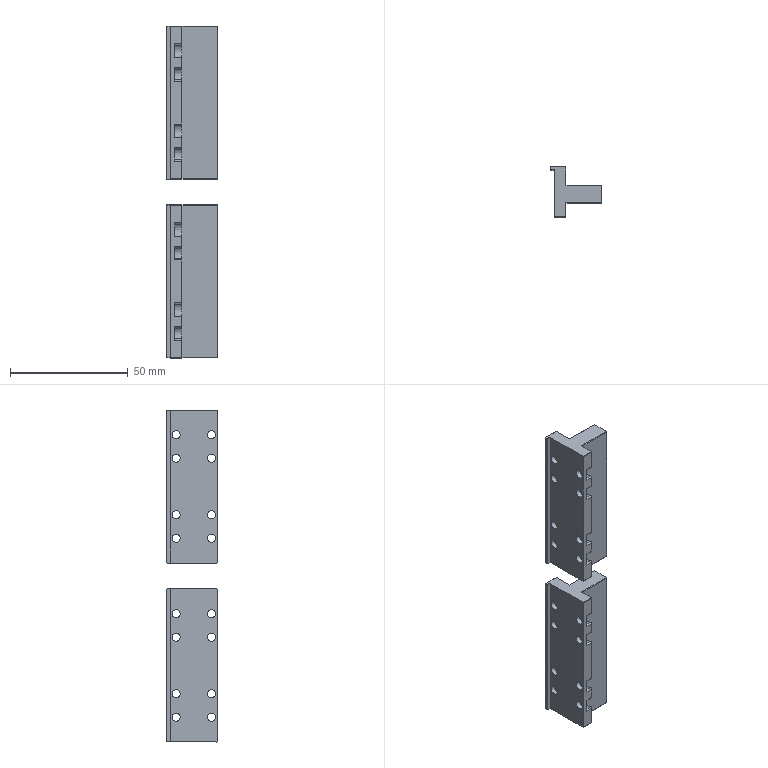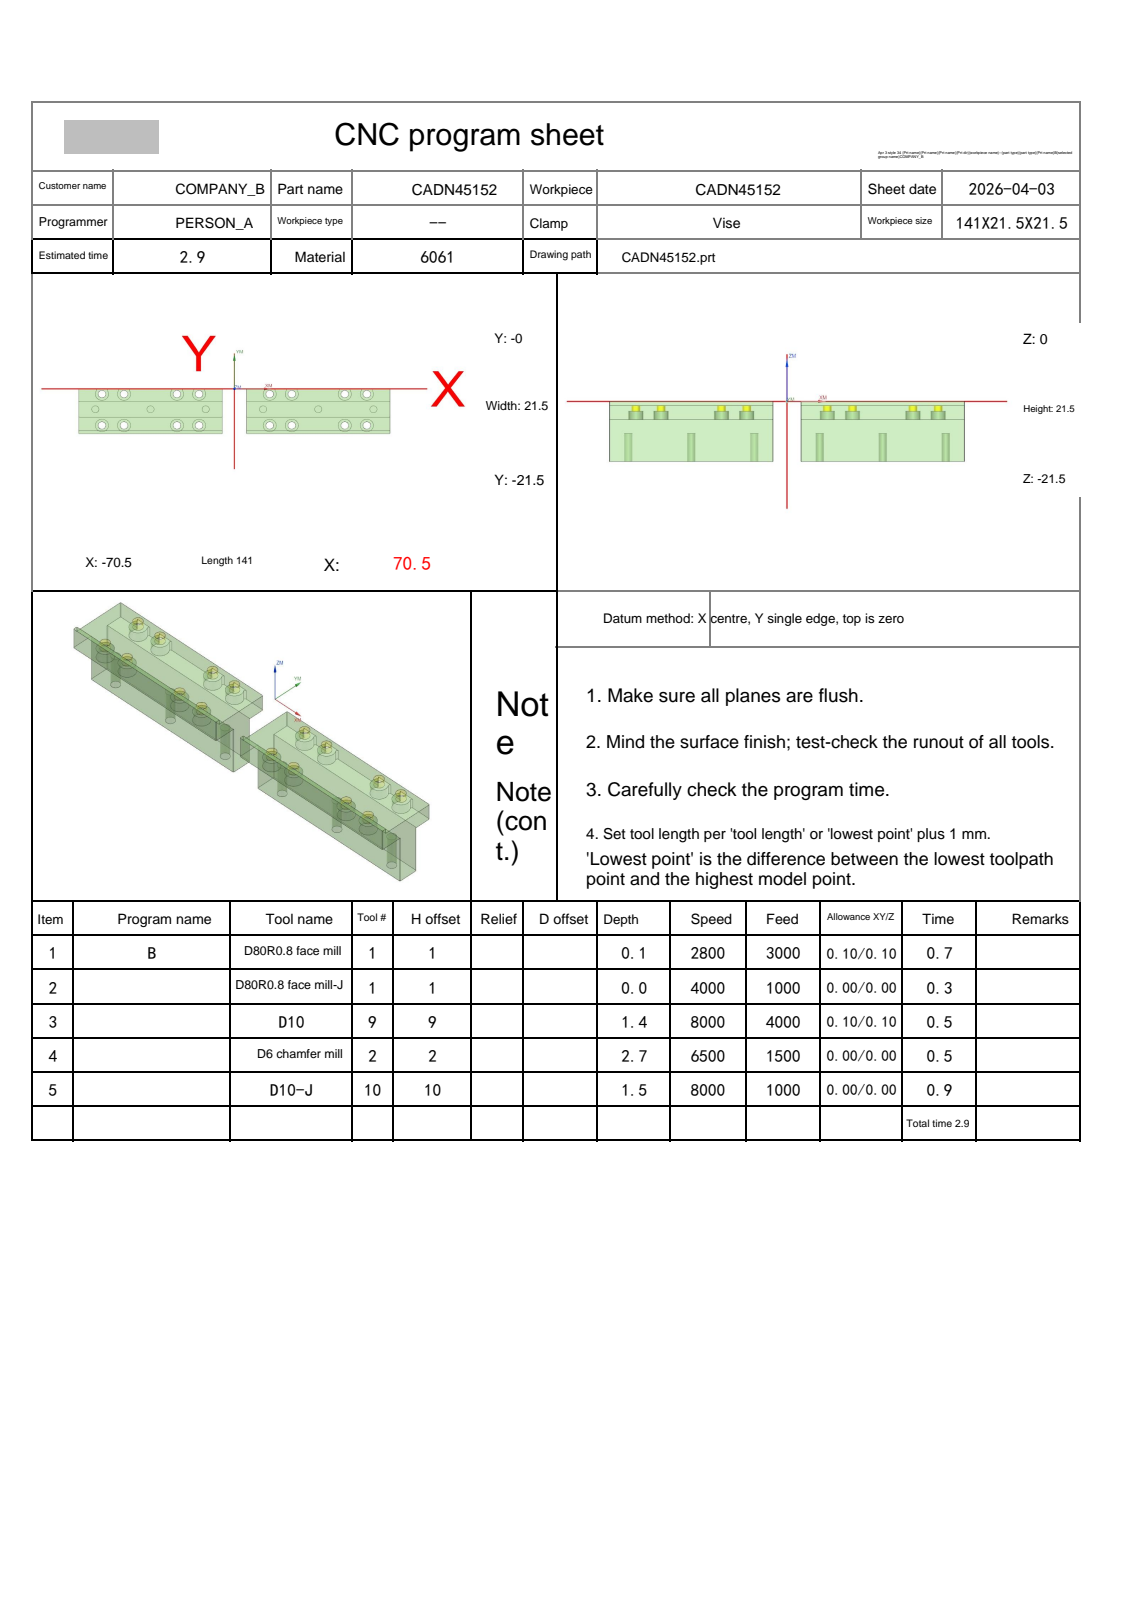NC program | NX | posted by the shop | part box 21.5 x 21.5 x 141 mm
Whole program:
%
O0001
(Machine time: 3.90 MIN)
(===Total Tool:4===)
(T1=D80R0.8 face mill D=80.  R=0.8  D-  H01 Z=0.    )
(T9=D10     D=10.  R=0.   D-  H09 Z=-1.4  )
(T2=D6 chamfer mill   D=6.   R=0.   D-  H02 Z=-2.7  )
(T10=D10-J  D=10.  R=0.   D10 H10 Z=-1.5  )
G80 G90 G17 G49 G40
G91 G28 Z0
M01
N1 T01 M06
(D80R0.8 face mill  D=80. R=0.8 H=01 ce=0.10 di=0.10)
G00 G90 G54 X122.597 Y-10.75 M03 S2800
G43 H01 Z20.
M08
Z5.014
G01 Z3.014 F3000.
X110.597
X-110.597
X-122.597
Z5.014
G00 X122.597
Z4.529
G01 Z2.529
X110.597
X-110.597
X-122.597
Z4.529
G00 X122.597
Z4.043
G01 Z2.043
X110.597
X-110.597
X-122.597
Z4.043
G00 X122.597
Z3.557
G01 Z1.557
X110.597
X-110.597
X-122.597
Z3.557
G00 Z20.
X122.597
Z3.071
G01 Z1.071
X110.597
X-110.597
X-122.597
Z3.071
G00 Z20.
X122.597
Z2.586
G01 Z.586
X110.597
X-110.597
X-122.597
Z2.586
G00 Z20.
X122.597
Z2.1
G01 Z.1
X110.597
X-110.597
X-122.597
Z2.1
G00 Z20.
G91 G28 Z0.0
M05
M09
G91 G28 Z0.0
M01
N2 T01 M06
(D80R0.8 face mill-J  D=80. R=0.8 H=01 ce=0.00 di=0.00)
G00 G90 G54 X122.499 Y-10.736 M03 S4000
G43 H01 Z20.
M08
Z2.
G01 Z0.0 F1000.
X110.499 Y-10.737
X-110.499 Y-10.763
X-122.499 Y-10.764
Z2.
G00 Z20.
G91 G28 Z0.0
M05
M09
G91 G28 Z0.0
M01
N3 T09 M06
(D10  D=10. R=0. H=09 ce=0.10 di=0.10)
G00 G90 G54 X0.0 Y8. M03 S8000
G43 H09 Z13.3
M08
Z1.033
G01 Z-.467 F4000.
Y4.9
X72.33
X75.4 Y1.83
Y-14.9
X-72.412
X-75.4 Y-17.888
Y1.83
X-72.33 Y4.9
X-3.035
G02 X-2.203 Y4.455 I-.001 J-1.
G01 X2.203 Y-2.155
G03 X3.035 Y-2.6 I.832 J.555
G01 X66.904
G02 X67.9 Y-3.596 I-.004 J-1.
G01 Y-6.404
G02 X66.904 Y-7.4 I-1. J.004
G01 X-66.904
G02 X-67.9 Y-6.404 I.004 J1.
G01 Y-3.596
G02 X-66.904 Y-2.6 I1. J-.004
G01 X0.0
X.5
Y.4
Y8.
Z1.033
G00 X0.0
Z.567
G01 Z-.933
Y4.9
X72.33
X75.4 Y1.83
Y-14.9
X-72.412
X-75.4 Y-17.888
Y1.83
X-72.33 Y4.9
X-3.035
G02 X-2.203 Y4.455 I-.001 J-1.
G01 X2.203 Y-2.155
G03 X3.035 Y-2.6 I.832 J.555
G01 X66.904
G02 X67.9 Y-3.596 I-.004 J-1.
G01 Y-6.404
G02 X66.904 Y-7.4 I-1. J.004
G01 X-66.904
G02 X-67.9 Y-6.404 I.004 J1.
G01 Y-3.596
G02 X-66.904 Y-2.6 I1. J-.004
G01 X0.0
X.5
Y.4
Y8.
Z.567
G00 X0.0
Z.1
G01 Z-1.4
Y4.9
X72.33
X75.4 Y1.83
Y-14.9
X-72.412
X-75.4 Y-17.888
Y1.83
X-72.33 Y4.9
X-3.035
G02 X-2.203 Y4.455 I-.001 J-1.
G01 X2.203 Y-2.155
G03 X3.035 Y-2.6 I.832 J.555
G01 X66.904
G02 X67.9 Y-3.596 I-.004 J-1.
G01 Y-6.404
G02 X66.904 Y-7.4 I-1. J.004
G01 X-66.904
G02 X-67.9 Y-6.404 I.004 J1.
G01 Y-3.596
G02 X-66.904 Y-2.6 I1. J-.004
G01 X0.0
X.5
Y.4
Y8.
Z.1
G00 Z13.3
G91 G28 Z0.0
M05
M09
G91 G28 Z0.0
M01
N4 T02 M06
(D6 chamfer mill  D=6. R=0. H=02 ce=0.00 di=0.00)
G00 G90 G54 X37.714 Y-18.773 M03 S6500
G43 H02 Z20.
M08
Z.172
G01 Z-1.2 F1500.
G03 X38. Y-18.973 I1.286 J1.532
G01 X38.046 Y-19.003
X38.1 Y-19.
X70.5
G02 X71.5 Y-20. I0.0 J-1.
G01 Y-21.3
X71.466 Y-21.559
X71.366 Y-21.8
X71.207 Y-22.007
X71.007 Y-22.207
X70.8 Y-22.366
X70.559 Y-22.466
X70.3 Y-22.5
X5.7
X5.441 Y-22.466
X5.2 Y-22.366
X4.993 Y-22.207
X4.793 Y-22.007
X4.634 Y-21.8
X4.534 Y-21.559
X4.5 Y-21.3
Y-20.2
X4.534 Y-19.941
X4.634 Y-19.7
X4.793 Y-19.493
X4.993 Y-19.293
X5.2 Y-19.134
X5.441 Y-19.034
X5.7 Y-19.
X38.1
X38.154 Y-19.003
X38.2 Y-18.973
G03 X38.486 Y-18.773 I-1. J1.732
G01 Z.172
G00 Z10.
X-38.286
Z.172
G01 Z-1.2
G03 X-38. Y-18.973 I1.286 J1.532
G01 X-37.954 Y-19.003
X-37.9 Y-19.
X-5.5
G02 X-4.5 Y-20. I0.0 J-1.
G01 Y-21.3
X-4.534 Y-21.559
X-4.634 Y-21.8
X-4.793 Y-22.007
X-4.993 Y-22.207
X-5.2 Y-22.366
X-5.441 Y-22.466
X-5.7 Y-22.5
X-70.3
X-70.559 Y-22.466
X-70.8 Y-22.366
X-71.007 Y-22.207
X-71.207 Y-22.007
X-71.366 Y-21.8
X-71.466 Y-21.559
X-71.5 Y-21.3
Y-20.2
X-71.466 Y-19.941
X-71.366 Y-19.7
X-71.207 Y-19.493
X-71.007 Y-19.293
X-70.8 Y-19.134
X-70.559 Y-19.034
X-70.3 Y-19.
X-37.9
X-37.846 Y-19.003
X-37.8 Y-18.973
G03 X-37.514 Y-18.773 I-1. J1.732
G01 Z.172
G00 Z10.
X-71.5 Y-17.583
Z1.3
G01 Z-2.7
Y-.2
X-71.466 Y.059
X-71.366 Y.3
X-71.207 Y.507
X-71.007 Y.707
X-70.8 Y.866
X-70.559 Y.966
X-70.3 Y1.
X-5.7
X-5.441 Y.966
X-5.2 Y.866
X-4.993 Y.707
X-4.793 Y.507
X-4.634 Y.3
X-4.534 Y.059
X-4.5 Y-.2
Y-17.486
Z1.3
G00 Z10.
X-16.576 Y-2.088
Z-1.137
G01 Z-2.7
G03 X-16.736 Y-2.397 I1.687 J-1.075
G01 X-16.76 Y-2.446
X-16.75 Y-2.5
G03 X-16. Y-3.25 I.75 J0.0
X-15.25 Y-2.5 I0.0 J.75
X-16. Y-1.75 I-.75 J0.0
X-16.724 Y-2.306 I0.0 J-.75
G01 X-16.75 Y-2.5
X-16.76 Y-2.554
X-16.736 Y-2.603
G03 X-16.576 Y-2.912 I1.848 J.765
G01 Z-1.137
G00 Z1.05
X-26.576 Y-2.088
Z-1.137
G01 Z-2.7
G03 X-26.736 Y-2.397 I1.687 J-1.075
G01 X-26.76 Y-2.446
X-26.75 Y-2.5
G03 X-26. Y-3.25 I.75 J0.0
X-25.25 Y-2.5 I0.0 J.75
X-26. Y-1.75 I-.75 J0.0
X-26.724 Y-2.306 I0.0 J-.75
G01 X-26.75 Y-2.5
X-26.76 Y-2.554
X-26.736 Y-2.603
G03 X-26.576 Y-2.912 I1.848 J.765
G01 Z-1.137
G00 Z10.
X-15.279 Y-17.307
Z1.3
G01 Z-2.7
X-15.283 Y-17.279
G03 X-16. Y-16.75 I-.717 J-.221
X-16.53 Y-16.97 I0.0 J-.75
G01 X-16.65 Y-17.125
X-16.724 Y-17.306
Z1.3
G00 X-25.279 Y-17.307
G01 Z-2.7
X-25.283 Y-17.279
G03 X-26. Y-16.75 I-.717 J-.221
X-26.53 Y-16.97 I0.0 J-.75
G01 X-26.65 Y-17.125
X-26.724 Y-17.306
Z1.3
G00 Z10.
X-49.279 Y-17.307
Z1.3
G01 Z-2.7
X-49.283 Y-17.279
G03 X-50. Y-16.75 I-.717 J-.221
X-50.53 Y-16.97 I0.0 J-.75
G01 X-50.65 Y-17.125
X-50.724 Y-17.306
Z1.3
G00 X-59.279 Y-17.307
G01 Z-2.7
X-59.283 Y-17.279
G03 X-60. Y-16.75 I-.717 J-.221
X-60.53 Y-16.97 I0.0 J-.75
G01 X-60.65 Y-17.125
X-60.724 Y-17.306
Z1.3
G00 Z10.
X-60.576 Y-2.088
Z-1.137
G01 Z-2.7
G03 X-60.736 Y-2.397 I1.687 J-1.075
G01 X-60.76 Y-2.446
X-60.75 Y-2.5
G03 X-60. Y-3.25 I.75 J0.0
X-59.25 Y-2.5 I0.0 J.75
X-60. Y-1.75 I-.75 J0.0
X-60.724 Y-2.306 I0.0 J-.75
G01 X-60.75 Y-2.5
X-60.76 Y-2.554
X-60.736 Y-2.603
G03 X-60.576 Y-2.912 I1.848 J.765
G01 Z-1.137
G00 Z1.05
X-50.576 Y-2.088
Z-1.137
G01 Z-2.7
G03 X-50.736 Y-2.397 I1.687 J-1.075
G01 X-50.76 Y-2.446
X-50.75 Y-2.5
G03 X-50. Y-3.25 I.75 J0.0
X-49.25 Y-2.5 I0.0 J.75
X-50. Y-1.75 I-.75 J0.0
X-50.724 Y-2.306 I0.0 J-.75
G01 X-50.75 Y-2.5
X-50.76 Y-2.554
X-50.736 Y-2.603
G03 X-50.576 Y-2.912 I1.848 J.765
G01 Z-1.137
G00 Z10.
X4.5 Y-17.583
Z1.3
G01 Z-2.7
Y-.2
X4.534 Y.059
X4.634 Y.3
X4.793 Y.507
X4.993 Y.707
X5.2 Y.866
X5.441 Y.966
X5.7 Y1.
X70.3
X70.559 Y.966
X70.8 Y.866
X71.007 Y.707
X71.207 Y.507
X71.366 Y.3
X71.466 Y.059
X71.5 Y-.2
Y-17.486
Z1.3
G00 Z10.
X59.424 Y-2.088
Z-1.137
G01 Z-2.7
G03 X59.264 Y-2.397 I1.687 J-1.075
G01 X59.24 Y-2.446
X59.25 Y-2.5
G03 X60. Y-3.25 I.75 J0.0
X60.75 Y-2.5 I0.0 J.75
X60. Y-1.75 I-.75 J0.0
X59.276 Y-2.306 I0.0 J-.75
G01 X59.25 Y-2.5
X59.24 Y-2.554
X59.264 Y-2.603
G03 X59.424 Y-2.912 I1.848 J.765
G01 Z-1.137
G00 Z1.05
X49.424 Y-2.088
Z-1.137
G01 Z-2.7
G03 X49.264 Y-2.397 I1.687 J-1.075
G01 X49.24 Y-2.446
X49.25 Y-2.5
G03 X50. Y-3.25 I.75 J0.0
X50.75 Y-2.5 I0.0 J.75
X50. Y-1.75 I-.75 J0.0
X49.276 Y-2.306 I0.0 J-.75
G01 X49.25 Y-2.5
X49.24 Y-2.554
X49.264 Y-2.603
G03 X49.424 Y-2.912 I1.848 J.765
G01 Z-1.137
G00 Z10.
X60.721 Y-17.307
Z1.3
G01 Z-2.7
X60.717 Y-17.279
G03 X60. Y-16.75 I-.717 J-.221
X59.47 Y-16.97 I0.0 J-.75
G01 X59.35 Y-17.125
X59.276 Y-17.306
Z1.3
G00 X50.721 Y-17.307
G01 Z-2.7
X50.717 Y-17.279
G03 X50. Y-16.75 I-.717 J-.221
X49.47 Y-16.97 I0.0 J-.75
G01 X49.35 Y-17.125
X49.276 Y-17.306
Z1.3
G00 Z10.
X26.721 Y-17.307
Z1.3
G01 Z-2.7
X26.717 Y-17.279
G03 X26. Y-16.75 I-.717 J-.221
X25.47 Y-16.97 I0.0 J-.75
G01 X25.35 Y-17.125
X25.276 Y-17.306
Z1.3
G00 X16.721 Y-17.307
G01 Z-2.7
X16.717 Y-17.279
G03 X16. Y-16.75 I-.717 J-.221
X15.47 Y-16.97 I0.0 J-.75
G01 X15.35 Y-17.125
X15.276 Y-17.306
Z1.3
G00 Z10.
X15.424 Y-2.088
Z-1.137
G01 Z-2.7
G03 X15.264 Y-2.397 I1.687 J-1.075
G01 X15.24 Y-2.446
X15.25 Y-2.5
G03 X16. Y-3.25 I.75 J0.0
X16.75 Y-2.5 I0.0 J.75
X16. Y-1.75 I-.75 J0.0
X15.276 Y-2.306 I0.0 J-.75
G01 X15.25 Y-2.5
X15.24 Y-2.554
X15.264 Y-2.603
G03 X15.424 Y-2.912 I1.848 J.765
G01 Z-1.137
G00 Z1.05
X25.424 Y-2.088
Z-1.137
G01 Z-2.7
G03 X25.264 Y-2.397 I1.687 J-1.075
G01 X25.24 Y-2.446
X25.25 Y-2.5
G03 X26. Y-3.25 I.75 J0.0
X26.75 Y-2.5 I0.0 J.75
X26. Y-1.75 I-.75 J0.0
X25.276 Y-2.306 I0.0 J-.75
G01 X25.25 Y-2.5
X25.24 Y-2.554
X25.264 Y-2.603
G03 X25.424 Y-2.912 I1.848 J.765
G01 Z-1.137
G00 Z20.
G91 G28 Z0.0
M05
M09
G91 G28 Z0.0
M01
N5 T10 M06
(D10-J  D=10. R=0. H=10 ce=0.40 di=0.00)
G00 G90 G54 X-77.419 Y2.436 M03 S8000
G43 H10 Z13.3
M08
Z0.0
G01 Z-1.5 F1000.
G03 X-75.5 Y1. I1.919 J.564
G01 X74.6
G02 X75.5 Y.1 I0.0 J-.9
G01 Y-1.9
G02 X74.5 Y-2.9 I-1. J0.0
G01 X-74.6
G03 X-75.5 Y-3.8 I0.0 J-.9
G01 Y-5.8
G03 X-74.5 Y-6.8 I1. J0.0
G01 X74.6
G02 X75.5 Y-7.7 I0.0 J-.9
G01 Y-9.7
G02 X74.5 Y-10.7 I-1. J0.0
G01 X-74.6
G03 X-75.5 Y-11.6 I0.0 J-.9
G01 Y-13.6
G03 X-74.5 Y-14.6 I1. J0.0
G01 X75.5
G03 X77.5 Y-12.6 I0.0 J2.
G01 Z0.0
G00 Z13.3
G00 G90 X-77.691 Y-18.568 M03 S8000
Z13.3
Z-.5
G01 Z-1.5 F1000.
G41 D10
X-77.5 Y-18.627
G03 X-76.914 Y-18.715 I.586 J1.912
X-75.5 Y-18.129 I0.0 J2.
G01 X-72.371 Y-15.
X75.5
G03 X77.5 Y-13.001 I0.0 J2.
G01 G40 Y-12.801
Z-.5
G00 Z13.3
M05
M09
G91 G28 Z0.0
G91 G28 Y0.0
M30
%